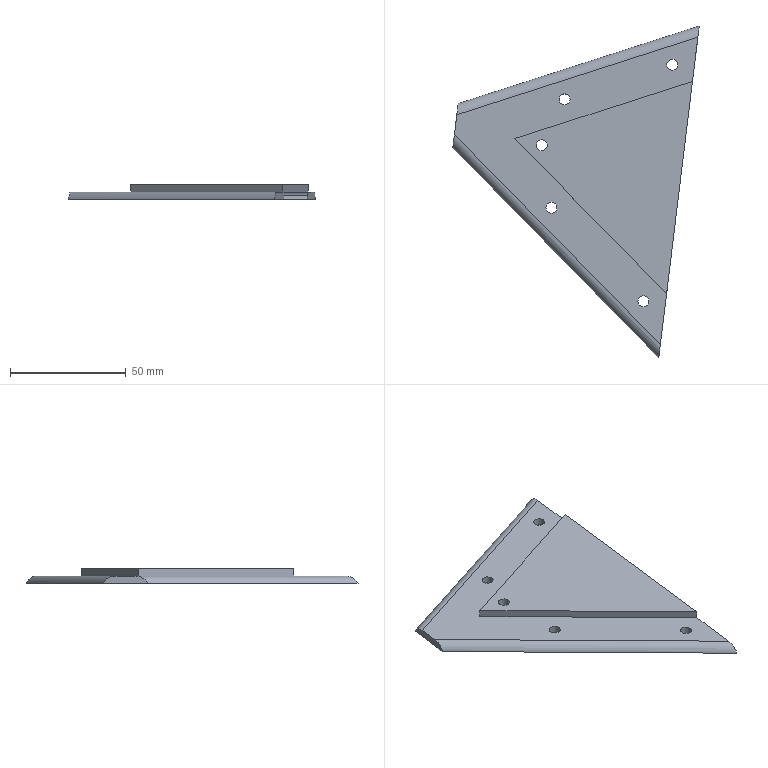Part | NX | features MG0301 nose pivot 24(left) 2 | 1 solid | 25 faces | box 106.679 x 143.723 x 6.35 mm | volume 27507 mm3 | cylinder 12 | plane 11 | torus 2 | commonest cylinder face diameters 4.763 x5 3.15 x3 9.525 x2 12.7 x2
STEP:
#1=CARTESIAN_POINT('',(-353.678,-108.911,-6.35));
#2=VERTEX_POINT('',#1);
#3=CARTESIAN_POINT('',(-354.276,-113.821,-3.175));
#4=VERTEX_POINT('',#3);
#5=CARTESIAN_POINT('',(-354.276,-113.821,-7.938));
#6=DIRECTION('',(-0.9927,0.1209,0.));
#7=DIRECTION('',(0.1209,0.9927,0.));
#8=AXIS2_PLACEMENT_3D('',#5,#6,#7);
#9=ELLIPSE('',#8,5.246,4.763);
#10=EDGE_CURVE('',#2,#4,#9,.F.);
#11=ORIENTED_EDGE('',*,*,#10,.F.);
#12=CARTESIAN_POINT('',(-356.021,-128.145,-6.35));
#13=VERTEX_POINT('',#12);
#14=CARTESIAN_POINT('',(-353.219,-105.142,-6.35));
#15=DIRECTION('',(-0.1209,-0.9927,0.));
#16=VECTOR('',#15,1000.);
#17=LINE('',#14,#16);
#18=EDGE_CURVE('',#2,#13,#17,.T.);
#19=ORIENTED_EDGE('',*,*,#18,.T.);
#20=CARTESIAN_POINT('',(-355.326,-122.441,-3.175));
#21=VERTEX_POINT('',#20);
#22=CARTESIAN_POINT('',(-355.326,-122.441,-7.938));
#23=DIRECTION('',(-0.9927,0.1209,0.));
#24=DIRECTION('',(0.1209,0.9927,0.));
#25=AXIS2_PLACEMENT_3D('',#22,#23,#24);
#26=ELLIPSE('',#25,6.095,4.763);
#27=EDGE_CURVE('',#21,#13,#26,.F.);
#28=ORIENTED_EDGE('',*,*,#27,.F.);
#29=CARTESIAN_POINT('',(-353.219,-105.142,-3.175));
#30=DIRECTION('',(-0.1209,-0.9927,0.));
#31=VECTOR('',#30,1000.);
#32=LINE('',#29,#31);
#33=EDGE_CURVE('',#4,#21,#32,.T.);
#34=ORIENTED_EDGE('',*,*,#33,.F.);
#35=EDGE_LOOP('',(#11,#19,#28,#34));
#36=FACE_BOUND('',#35,.T.);
#37=CARTESIAN_POINT('',(-353.219,-105.142,-6.35));
#38=DIRECTION('',(-0.9927,0.1209,0.));
#39=DIRECTION('',(-0.1209,-0.9927,0.));
#40=AXIS2_PLACEMENT_3D('',#37,#38,#39);
#41=PLANE('',#40);
#42=ADVANCED_FACE('',(#36),#41,.T.);
#43=CARTESIAN_POINT('',(-249.941,-80.241,-3.175));
#44=VERTEX_POINT('',#43);
#45=CARTESIAN_POINT('',(-249.343,-75.332,-6.35));
#46=VERTEX_POINT('',#45);
#47=CARTESIAN_POINT('',(-249.941,-80.241,-7.938));
#48=DIRECTION('',(0.9927,-0.1209,0.));
#49=DIRECTION('',(0.1209,0.9927,0.));
#50=AXIS2_PLACEMENT_3D('',#47,#48,#49);
#51=ELLIPSE('',#50,5.246,4.763);
#52=EDGE_CURVE('',#44,#46,#51,.F.);
#53=ORIENTED_EDGE('',*,*,#52,.F.);
#54=CARTESIAN_POINT('',(-252.267,-99.334,-3.175));
#55=VERTEX_POINT('',#54);
#56=CARTESIAN_POINT('',(-248.883,-71.562,-3.175));
#57=DIRECTION('',(0.1209,0.9927,0.));
#58=VECTOR('',#57,1000.);
#59=LINE('',#56,#58);
#60=EDGE_CURVE('',#55,#44,#59,.T.);
#61=ORIENTED_EDGE('',*,*,#60,.F.);
#62=CARTESIAN_POINT('',(-252.267,-99.334,0.));
#63=VERTEX_POINT('',#62);
#64=CARTESIAN_POINT('',(-252.267,-99.334,-6.35));
#65=DIRECTION('',(0.,0.,-1.));
#66=VECTOR('',#65,1000.);
#67=LINE('',#64,#66);
#68=EDGE_CURVE('',#63,#55,#67,.T.);
#69=ORIENTED_EDGE('',*,*,#68,.F.);
#70=CARTESIAN_POINT('',(-263.456,-191.168,0.));
#71=VERTEX_POINT('',#70);
#72=CARTESIAN_POINT('',(-248.883,-71.562,0.));
#73=DIRECTION('',(0.1209,0.9927,0.));
#74=VECTOR('',#73,1000.);
#75=LINE('',#72,#74);
#76=EDGE_CURVE('',#71,#63,#75,.T.);
#77=ORIENTED_EDGE('',*,*,#76,.F.);
#78=CARTESIAN_POINT('',(-263.456,-191.168,-3.175));
#79=VERTEX_POINT('',#78);
#80=CARTESIAN_POINT('',(-263.456,-191.168,-6.35));
#81=DIRECTION('',(0.,0.,1.));
#82=VECTOR('',#81,1000.);
#83=LINE('',#80,#82);
#84=EDGE_CURVE('',#79,#71,#83,.T.);
#85=ORIENTED_EDGE('',*,*,#84,.F.);
#86=CARTESIAN_POINT('',(-266.158,-213.351,-3.175));
#87=VERTEX_POINT('',#86);
#88=CARTESIAN_POINT('',(-248.883,-71.562,-3.175));
#89=DIRECTION('',(0.1209,0.9927,0.));
#90=VECTOR('',#89,1000.);
#91=LINE('',#88,#90);
#92=EDGE_CURVE('',#87,#79,#91,.T.);
#93=ORIENTED_EDGE('',*,*,#92,.F.);
#94=CARTESIAN_POINT('',(-266.853,-219.055,-6.35));
#95=VERTEX_POINT('',#94);
#96=CARTESIAN_POINT('',(-266.158,-213.351,-7.938));
#97=DIRECTION('',(0.9927,-0.1209,0.));
#98=DIRECTION('',(0.1209,0.9927,0.));
#99=AXIS2_PLACEMENT_3D('',#96,#97,#98);
#100=ELLIPSE('',#99,6.095,4.763);
#101=EDGE_CURVE('',#95,#87,#100,.F.);
#102=ORIENTED_EDGE('',*,*,#101,.F.);
#103=CARTESIAN_POINT('',(-262.964,-187.135,-6.35));
#104=VERTEX_POINT('',#103);
#105=CARTESIAN_POINT('',(-248.883,-71.562,-6.35));
#106=DIRECTION('',(0.1209,0.9927,0.));
#107=VECTOR('',#106,1000.);
#108=LINE('',#105,#107);
#109=EDGE_CURVE('',#95,#104,#108,.T.);
#110=ORIENTED_EDGE('',*,*,#109,.T.);
#111=CARTESIAN_POINT('',(-262.964,-187.135,-4.75));
#112=VERTEX_POINT('',#111);
#113=CARTESIAN_POINT('',(-262.964,-187.135,-22.225));
#114=DIRECTION('',(0.,0.,1.));
#115=VECTOR('',#114,1000.);
#116=LINE('',#113,#115);
#117=EDGE_CURVE('',#104,#112,#116,.T.);
#118=ORIENTED_EDGE('',*,*,#117,.T.);
#119=CARTESIAN_POINT('',(-262.721,-185.135,-3.175));
#120=VERTEX_POINT('',#119);
#121=CARTESIAN_POINT('',(-262.721,-185.135,-4.75));
#122=DIRECTION('',(0.9927,-0.1209,0.));
#123=DIRECTION('',(-0.1209,-0.9927,0.));
#124=AXIS2_PLACEMENT_3D('',#121,#122,#123);
#125=ELLIPSE('',#124,2.015,1.575);
#126=EDGE_CURVE('',#112,#120,#125,.F.);
#127=ORIENTED_EDGE('',*,*,#126,.T.);
#128=CARTESIAN_POINT('',(-252.9,-104.528,-3.175));
#129=VERTEX_POINT('',#128);
#130=CARTESIAN_POINT('',(-252.69,-102.806,-3.175));
#131=DIRECTION('',(0.1209,0.9927,0.));
#132=VECTOR('',#131,1000.);
#133=LINE('',#130,#132);
#134=EDGE_CURVE('',#120,#129,#133,.T.);
#135=ORIENTED_EDGE('',*,*,#134,.T.);
#136=CARTESIAN_POINT('',(-252.69,-102.806,-4.75));
#137=VERTEX_POINT('',#136);
#138=CARTESIAN_POINT('',(-252.9,-104.528,-4.75));
#139=DIRECTION('',(0.9927,-0.1209,0.));
#140=DIRECTION('',(-0.1209,-0.9927,0.));
#141=AXIS2_PLACEMENT_3D('',#138,#139,#140);
#142=ELLIPSE('',#141,1.735,1.575);
#143=EDGE_CURVE('',#129,#137,#142,.F.);
#144=ORIENTED_EDGE('',*,*,#143,.T.);
#145=CARTESIAN_POINT('',(-252.69,-102.806,-6.35));
#146=VERTEX_POINT('',#145);
#147=CARTESIAN_POINT('',(-252.69,-102.806,-22.225));
#148=DIRECTION('',(0.,0.,1.));
#149=VECTOR('',#148,1000.);
#150=LINE('',#147,#149);
#151=EDGE_CURVE('',#146,#137,#150,.T.);
#152=ORIENTED_EDGE('',*,*,#151,.F.);
#153=CARTESIAN_POINT('',(-248.883,-71.562,-6.35));
#154=DIRECTION('',(0.1209,0.9927,0.));
#155=VECTOR('',#154,1000.);
#156=LINE('',#153,#155);
#157=EDGE_CURVE('',#146,#46,#156,.T.);
#158=ORIENTED_EDGE('',*,*,#157,.T.);
#159=EDGE_LOOP('',(#53,#61,#69,#77,#85,#93,#102,#110,#118,#127,#135,#144,#152,#158));
#160=FACE_BOUND('',#159,.T.);
#161=CARTESIAN_POINT('',(-248.883,-71.562,-6.35));
#162=DIRECTION('',(0.9927,-0.1209,0.));
#163=DIRECTION('',(0.1209,0.9927,0.));
#164=AXIS2_PLACEMENT_3D('',#161,#162,#163);
#165=PLANE('',#164);
#166=ADVANCED_FACE('',(#160),#165,.T.);
#167=CARTESIAN_POINT('',(-305.21,-107.134,-6.35));
#168=VERTEX_POINT('',#167);
#169=CARTESIAN_POINT('',(-307.591,-107.134,-6.35));
#170=DIRECTION('',(0.,0.,1.));
#171=DIRECTION('',(1.,0.,0.));
#172=AXIS2_PLACEMENT_3D('',#169,#170,#171);
#173=CIRCLE('',#172,2.381);
#174=EDGE_CURVE('',#168,#168,#173,.T.);
#175=ORIENTED_EDGE('',*,*,#174,.T.);
#176=EDGE_LOOP('',(#175));
#177=FACE_BOUND('',#176,.T.);
#178=CARTESIAN_POINT('',(-258.604,-92.134,-6.35));
#179=VERTEX_POINT('',#178);
#180=CARTESIAN_POINT('',(-260.985,-92.134,-6.35));
#181=DIRECTION('',(0.,0.,1.));
#182=DIRECTION('',(1.,0.,0.));
#183=AXIS2_PLACEMENT_3D('',#180,#181,#182);
#184=CIRCLE('',#183,2.381);
#185=EDGE_CURVE('',#179,#179,#184,.T.);
#186=ORIENTED_EDGE('',*,*,#185,.T.);
#187=EDGE_LOOP('',(#186));
#188=FACE_BOUND('',#187,.T.);
#189=CARTESIAN_POINT('',(-310.915,-153.957,-6.35));
#190=VERTEX_POINT('',#189);
#191=CARTESIAN_POINT('',(-313.296,-153.957,-6.35));
#192=DIRECTION('',(0.,0.,1.));
#193=DIRECTION('',(1.,0.,0.));
#194=AXIS2_PLACEMENT_3D('',#191,#192,#193);
#195=CIRCLE('',#194,2.381);
#196=EDGE_CURVE('',#190,#190,#195,.T.);
#197=ORIENTED_EDGE('',*,*,#196,.T.);
#198=EDGE_LOOP('',(#197));
#199=FACE_BOUND('',#198,.T.);
#200=CARTESIAN_POINT('',(-271.084,-194.566,-6.35));
#201=VERTEX_POINT('',#200);
#202=CARTESIAN_POINT('',(-273.465,-194.566,-6.35));
#203=DIRECTION('',(0.,0.,1.));
#204=DIRECTION('',(1.,0.,0.));
#205=AXIS2_PLACEMENT_3D('',#202,#203,#204);
#206=CIRCLE('',#205,2.381);
#207=EDGE_CURVE('',#201,#201,#206,.T.);
#208=ORIENTED_EDGE('',*,*,#207,.T.);
#209=EDGE_LOOP('',(#208));
#210=FACE_BOUND('',#209,.T.);
#211=CARTESIAN_POINT('',(-315.119,-127.,-6.35));
#212=VERTEX_POINT('',#211);
#213=CARTESIAN_POINT('',(-317.5,-127.,-6.35));
#214=DIRECTION('',(0.,0.,1.));
#215=DIRECTION('',(1.,0.,0.));
#216=AXIS2_PLACEMENT_3D('',#213,#214,#215);
#217=CIRCLE('',#216,2.381);
#218=EDGE_CURVE('',#212,#212,#217,.T.);
#219=ORIENTED_EDGE('',*,*,#218,.T.);
#220=EDGE_LOOP('',(#219));
#221=FACE_BOUND('',#220,.T.);
#222=ORIENTED_EDGE('',*,*,#18,.F.);
#223=CARTESIAN_POINT('',(-475.205,-148.024,-6.35));
#224=DIRECTION('',(0.9519,0.3064,0.));
#225=VECTOR('',#224,1000.);
#226=LINE('',#223,#225);
#227=EDGE_CURVE('',#2,#46,#226,.T.);
#228=ORIENTED_EDGE('',*,*,#227,.T.);
#229=ORIENTED_EDGE('',*,*,#157,.F.);
#230=CARTESIAN_POINT('',(-295.429,-116.561,-6.35));
#231=VERTEX_POINT('',#230);
#232=CARTESIAN_POINT('',(-344.464,-132.343,-6.35));
#233=DIRECTION('',(-0.9519,-0.3064,0.));
#234=VECTOR('',#233,1000.);
#235=LINE('',#232,#234);
#236=EDGE_CURVE('',#146,#231,#235,.T.);
#237=ORIENTED_EDGE('',*,*,#236,.T.);
#238=CARTESIAN_POINT('',(-299.787,-121.838,-6.35));
#239=VERTEX_POINT('',#238);
#240=CARTESIAN_POINT('',(-293.484,-122.606,-6.35));
#241=DIRECTION('',(0.,0.,1.));
#242=DIRECTION('',(1.,0.,0.));
#243=AXIS2_PLACEMENT_3D('',#240,#241,#242);
#244=CIRCLE('',#243,6.35);
#245=EDGE_CURVE('',#231,#239,#244,.T.);
#246=ORIENTED_EDGE('',*,*,#245,.T.);
#247=CARTESIAN_POINT('',(-302.426,-143.493,-6.35));
#248=VERTEX_POINT('',#247);
#249=CARTESIAN_POINT('',(-298.565,-111.801,-6.35));
#250=DIRECTION('',(-0.1209,-0.9927,0.));
#251=VECTOR('',#250,1000.);
#252=LINE('',#249,#251);
#253=EDGE_CURVE('',#239,#248,#252,.T.);
#254=ORIENTED_EDGE('',*,*,#253,.T.);
#255=CARTESIAN_POINT('',(-300.656,-148.708,-6.35));
#256=VERTEX_POINT('',#255);
#257=CARTESIAN_POINT('',(-296.122,-144.261,-6.35));
#258=DIRECTION('',(0.,0.,1.));
#259=DIRECTION('',(1.,0.,0.));
#260=AXIS2_PLACEMENT_3D('',#257,#258,#259);
#261=CIRCLE('',#260,6.35);
#262=EDGE_CURVE('',#248,#256,#261,.T.);
#263=ORIENTED_EDGE('',*,*,#262,.T.);
#264=CARTESIAN_POINT('',(-348.207,-100.227,-6.35));
#265=DIRECTION('',(0.7002,-0.7139,0.));
#266=VECTOR('',#265,1000.);
#267=LINE('',#264,#266);
#268=EDGE_CURVE('',#256,#104,#267,.T.);
#269=ORIENTED_EDGE('',*,*,#268,.T.);
#270=ORIENTED_EDGE('',*,*,#109,.F.);
#271=CARTESIAN_POINT('',(22.703,-514.268,-6.35));
#272=DIRECTION('',(-0.7002,0.7139,0.));
#273=VECTOR('',#272,1000.);
#274=LINE('',#271,#273);
#275=EDGE_CURVE('',#95,#13,#274,.T.);
#276=ORIENTED_EDGE('',*,*,#275,.T.);
#277=EDGE_LOOP('',(#222,#228,#229,#237,#246,#254,#263,#269,#270,#276));
#278=FACE_BOUND('',#277,.T.);
#279=CARTESIAN_POINT('',(-353.219,-105.142,-6.35));
#280=DIRECTION('',(0.,0.,1.));
#281=DIRECTION('',(1.,0.,0.));
#282=AXIS2_PLACEMENT_3D('',#279,#280,#281);
#283=PLANE('',#282);
#284=ADVANCED_FACE('',(#177,#188,#199,#210,#221,#278),#283,.F.);
#285=CARTESIAN_POINT('',(-329.234,-124.106,0.));
#286=VERTEX_POINT('',#285);
#287=CARTESIAN_POINT('',(-468.479,-168.921,0.));
#288=DIRECTION('',(0.9519,0.3064,0.));
#289=VECTOR('',#288,1000.);
#290=LINE('',#287,#289);
#291=EDGE_CURVE('',#286,#63,#290,.T.);
#292=ORIENTED_EDGE('',*,*,#291,.F.);
#293=CARTESIAN_POINT('',(-350.474,-102.45,0.));
#294=DIRECTION('',(-0.7002,0.7139,0.));
#295=VECTOR('',#294,1000.);
#296=LINE('',#293,#295);
#297=EDGE_CURVE('',#71,#286,#296,.T.);
#298=ORIENTED_EDGE('',*,*,#297,.F.);
#299=ORIENTED_EDGE('',*,*,#76,.T.);
#300=EDGE_LOOP('',(#292,#298,#299));
#301=FACE_BOUND('',#300,.T.);
#302=CARTESIAN_POINT('',(-315.119,-127.,0.));
#303=VERTEX_POINT('',#302);
#304=CARTESIAN_POINT('',(-317.5,-127.,0.));
#305=DIRECTION('',(0.,0.,1.));
#306=DIRECTION('',(1.,0.,0.));
#307=AXIS2_PLACEMENT_3D('',#304,#305,#306);
#308=CIRCLE('',#307,2.381);
#309=EDGE_CURVE('',#303,#303,#308,.T.);
#310=ORIENTED_EDGE('',*,*,#309,.F.);
#311=EDGE_LOOP('',(#310));
#312=FACE_BOUND('',#311,.T.);
#313=CARTESIAN_POINT('',(-353.219,-105.142,0.));
#314=DIRECTION('',(0.,0.,1.));
#315=DIRECTION('',(1.,0.,0.));
#316=AXIS2_PLACEMENT_3D('',#313,#314,#315);
#317=PLANE('',#316);
#318=ADVANCED_FACE('',(#301,#312),#317,.T.);
#319=ORIENTED_EDGE('',*,*,#218,.F.);
#320=EDGE_LOOP('',(#319));
#321=FACE_BOUND('',#320,.T.);
#322=ORIENTED_EDGE('',*,*,#309,.T.);
#323=EDGE_LOOP('',(#322));
#324=FACE_BOUND('',#323,.T.);
#325=CARTESIAN_POINT('',(-317.5,-127.,-6.35));
#326=DIRECTION('',(0.,0.,1.));
#327=DIRECTION('',(1.,0.,0.));
#328=AXIS2_PLACEMENT_3D('',#325,#326,#327);
#329=CYLINDRICAL_SURFACE('',#328,2.381);
#330=ADVANCED_FACE('',(#321,#324),#329,.F.);
#331=CARTESIAN_POINT('',(-300.656,-148.708,-4.75));
#332=VERTEX_POINT('',#331);
#333=CARTESIAN_POINT('',(-300.656,-148.708,-3.175));
#334=DIRECTION('',(0.,0.,1.));
#335=VECTOR('',#334,1000.);
#336=LINE('',#333,#335);
#337=EDGE_CURVE('',#256,#332,#336,.T.);
#338=ORIENTED_EDGE('',*,*,#337,.T.);
#339=CARTESIAN_POINT('',(-302.795,-146.526,-4.75));
#340=DIRECTION('',(0.7002,-0.7139,0.));
#341=VECTOR('',#340,1000.);
#342=LINE('',#339,#341);
#343=EDGE_CURVE('',#332,#112,#342,.T.);
#344=ORIENTED_EDGE('',*,*,#343,.T.);
#345=ORIENTED_EDGE('',*,*,#117,.F.);
#346=ORIENTED_EDGE('',*,*,#268,.F.);
#347=EDGE_LOOP('',(#338,#344,#345,#346));
#348=FACE_BOUND('',#347,.T.);
#349=CARTESIAN_POINT('',(-302.795,-146.526,-22.225));
#350=DIRECTION('',(-0.7139,-0.7002,0.));
#351=DIRECTION('',(0.7002,-0.7139,0.));
#352=AXIS2_PLACEMENT_3D('',#349,#350,#351);
#353=PLANE('',#352);
#354=ADVANCED_FACE('',(#348),#353,.F.);
#355=CARTESIAN_POINT('',(-299.787,-121.838,-4.75));
#356=VERTEX_POINT('',#355);
#357=CARTESIAN_POINT('',(-299.787,-121.838,-3.175));
#358=DIRECTION('',(0.,0.,1.));
#359=VECTOR('',#358,1000.);
#360=LINE('',#357,#359);
#361=EDGE_CURVE('',#239,#356,#360,.T.);
#362=ORIENTED_EDGE('',*,*,#361,.T.);
#363=CARTESIAN_POINT('',(-302.426,-143.493,-4.75));
#364=VERTEX_POINT('',#363);
#365=CARTESIAN_POINT('',(-299.296,-117.806,-4.75));
#366=DIRECTION('',(-0.1209,-0.9927,0.));
#367=VECTOR('',#366,1000.);
#368=LINE('',#365,#367);
#369=EDGE_CURVE('',#356,#364,#368,.T.);
#370=ORIENTED_EDGE('',*,*,#369,.T.);
#371=CARTESIAN_POINT('',(-302.426,-143.493,-6.35));
#372=DIRECTION('',(0.,0.,1.));
#373=VECTOR('',#372,1000.);
#374=LINE('',#371,#373);
#375=EDGE_CURVE('',#364,#248,#374,.F.);
#376=ORIENTED_EDGE('',*,*,#375,.T.);
#377=ORIENTED_EDGE('',*,*,#253,.F.);
#378=EDGE_LOOP('',(#362,#370,#376,#377));
#379=FACE_BOUND('',#378,.T.);
#380=CARTESIAN_POINT('',(-299.296,-117.806,-22.225));
#381=DIRECTION('',(-0.9927,0.1209,0.));
#382=DIRECTION('',(-0.1209,-0.9927,0.));
#383=AXIS2_PLACEMENT_3D('',#380,#381,#382);
#384=PLANE('',#383);
#385=ADVANCED_FACE('',(#379),#384,.F.);
#386=ORIENTED_EDGE('',*,*,#151,.T.);
#387=CARTESIAN_POINT('',(-295.429,-116.561,-4.75));
#388=VERTEX_POINT('',#387);
#389=CARTESIAN_POINT('',(-252.69,-102.806,-4.75));
#390=DIRECTION('',(-0.9519,-0.3064,0.));
#391=VECTOR('',#390,1000.);
#392=LINE('',#389,#391);
#393=EDGE_CURVE('',#137,#388,#392,.T.);
#394=ORIENTED_EDGE('',*,*,#393,.T.);
#395=CARTESIAN_POINT('',(-295.429,-116.561,-6.35));
#396=DIRECTION('',(0.,0.,1.));
#397=VECTOR('',#396,1000.);
#398=LINE('',#395,#397);
#399=EDGE_CURVE('',#388,#231,#398,.F.);
#400=ORIENTED_EDGE('',*,*,#399,.T.);
#401=ORIENTED_EDGE('',*,*,#236,.F.);
#402=EDGE_LOOP('',(#386,#394,#400,#401));
#403=FACE_BOUND('',#402,.T.);
#404=CARTESIAN_POINT('',(-252.69,-102.806,-22.225));
#405=DIRECTION('',(-0.3064,0.9519,0.));
#406=DIRECTION('',(-0.9519,-0.3064,0.));
#407=AXIS2_PLACEMENT_3D('',#404,#405,#406);
#408=PLANE('',#407);
#409=ADVANCED_FACE('',(#403),#408,.F.);
#410=ORIENTED_EDGE('',*,*,#134,.F.);
#411=CARTESIAN_POINT('',(-299.531,-147.605,-3.175));
#412=VERTEX_POINT('',#411);
#413=CARTESIAN_POINT('',(-298.959,-148.188,-3.175));
#414=DIRECTION('',(0.7002,-0.7139,0.));
#415=VECTOR('',#414,1000.);
#416=LINE('',#413,#415);
#417=EDGE_CURVE('',#120,#412,#416,.F.);
#418=ORIENTED_EDGE('',*,*,#417,.T.);
#419=CARTESIAN_POINT('',(-300.863,-143.684,-3.175));
#420=VERTEX_POINT('',#419);
#421=CARTESIAN_POINT('',(-296.122,-144.261,-3.175));
#422=DIRECTION('',(0.,0.,-1.));
#423=DIRECTION('',(-1.,0.,0.));
#424=AXIS2_PLACEMENT_3D('',#421,#422,#423);
#425=CIRCLE('',#424,4.775);
#426=EDGE_CURVE('',#412,#420,#425,.T.);
#427=ORIENTED_EDGE('',*,*,#426,.T.);
#428=CARTESIAN_POINT('',(-298.224,-122.028,-3.175));
#429=VERTEX_POINT('',#428);
#430=CARTESIAN_POINT('',(-295.25,-97.62,-3.175));
#431=DIRECTION('',(-0.1209,-0.9927,0.));
#432=VECTOR('',#431,1000.);
#433=LINE('',#430,#432);
#434=EDGE_CURVE('',#420,#429,#433,.F.);
#435=ORIENTED_EDGE('',*,*,#434,.T.);
#436=CARTESIAN_POINT('',(-294.947,-118.06,-3.175));
#437=VERTEX_POINT('',#436);
#438=CARTESIAN_POINT('',(-293.484,-122.606,-3.175));
#439=DIRECTION('',(0.,0.,-1.));
#440=DIRECTION('',(-1.,0.,0.));
#441=AXIS2_PLACEMENT_3D('',#438,#439,#440);
#442=CIRCLE('',#441,4.775);
#443=EDGE_CURVE('',#429,#437,#442,.T.);
#444=ORIENTED_EDGE('',*,*,#443,.T.);
#445=CARTESIAN_POINT('',(-252.207,-104.305,-3.175));
#446=DIRECTION('',(-0.9519,-0.3064,0.));
#447=VECTOR('',#446,1000.);
#448=LINE('',#445,#447);
#449=EDGE_CURVE('',#437,#129,#448,.F.);
#450=ORIENTED_EDGE('',*,*,#449,.T.);
#451=EDGE_LOOP('',(#410,#418,#427,#435,#444,#450));
#452=FACE_BOUND('',#451,.T.);
#453=CARTESIAN_POINT('',(-252.69,-102.806,-3.175));
#454=DIRECTION('',(0.,0.,-1.));
#455=DIRECTION('',(-1.,0.,0.));
#456=AXIS2_PLACEMENT_3D('',#453,#454,#455);
#457=PLANE('',#456);
#458=ADVANCED_FACE('',(#452),#457,.T.);
#459=ORIENTED_EDGE('',*,*,#375,.F.);
#460=CARTESIAN_POINT('',(-296.122,-144.261,-4.75));
#461=DIRECTION('',(0.,0.,-1.));
#462=DIRECTION('',(-1.,0.,0.));
#463=AXIS2_PLACEMENT_3D('',#460,#461,#462);
#464=CIRCLE('',#463,6.35);
#465=EDGE_CURVE('',#364,#332,#464,.F.);
#466=ORIENTED_EDGE('',*,*,#465,.T.);
#467=ORIENTED_EDGE('',*,*,#337,.F.);
#468=ORIENTED_EDGE('',*,*,#262,.F.);
#469=EDGE_LOOP('',(#459,#466,#467,#468));
#470=FACE_BOUND('',#469,.T.);
#471=CARTESIAN_POINT('',(-296.122,-144.261,-22.225));
#472=DIRECTION('',(0.,0.,-1.));
#473=DIRECTION('',(-1.,0.,0.));
#474=AXIS2_PLACEMENT_3D('',#471,#472,#473);
#475=CYLINDRICAL_SURFACE('',#474,6.35);
#476=ADVANCED_FACE('',(#470),#475,.F.);
#477=ORIENTED_EDGE('',*,*,#399,.F.);
#478=CARTESIAN_POINT('',(-293.484,-122.606,-4.75));
#479=DIRECTION('',(0.,0.,-1.));
#480=DIRECTION('',(-1.,0.,0.));
#481=AXIS2_PLACEMENT_3D('',#478,#479,#480);
#482=CIRCLE('',#481,6.35);
#483=EDGE_CURVE('',#388,#356,#482,.F.);
#484=ORIENTED_EDGE('',*,*,#483,.T.);
#485=ORIENTED_EDGE('',*,*,#361,.F.);
#486=ORIENTED_EDGE('',*,*,#245,.F.);
#487=EDGE_LOOP('',(#477,#484,#485,#486));
#488=FACE_BOUND('',#487,.T.);
#489=CARTESIAN_POINT('',(-293.484,-122.606,-22.225));
#490=DIRECTION('',(0.,0.,-1.));
#491=DIRECTION('',(-1.,0.,0.));
#492=AXIS2_PLACEMENT_3D('',#489,#490,#491);
#493=CYLINDRICAL_SURFACE('',#492,6.35);
#494=ADVANCED_FACE('',(#488),#493,.F.);
#495=ORIENTED_EDGE('',*,*,#27,.T.);
#496=ORIENTED_EDGE('',*,*,#275,.F.);
#497=ORIENTED_EDGE('',*,*,#101,.T.);
#498=CARTESIAN_POINT('',(25.908,-511.124,-3.175));
#499=DIRECTION('',(-0.7002,0.7139,0.));
#500=VECTOR('',#499,1000.);
#501=LINE('',#498,#500);
#502=EDGE_CURVE('',#87,#21,#501,.T.);
#503=ORIENTED_EDGE('',*,*,#502,.T.);
#504=EDGE_LOOP('',(#495,#496,#497,#503));
#505=FACE_BOUND('',#504,.T.);
#506=CARTESIAN_POINT('',(25.908,-511.124,-7.938));
#507=DIRECTION('',(-0.7002,0.7139,0.));
#508=DIRECTION('',(-0.7139,-0.7002,0.));
#509=AXIS2_PLACEMENT_3D('',#506,#507,#508);
#510=CYLINDRICAL_SURFACE('',#509,4.763);
#511=ADVANCED_FACE('',(#505),#510,.T.);
#512=CARTESIAN_POINT('',(-309.973,-107.134,-3.175));
#513=VERTEX_POINT('',#512);
#514=CARTESIAN_POINT('',(-307.591,-107.134,-3.175));
#515=DIRECTION('',(0.,0.,-1.));
#516=DIRECTION('',(-1.,0.,0.));
#517=AXIS2_PLACEMENT_3D('',#514,#515,#516);
#518=CIRCLE('',#517,2.381);
#519=EDGE_CURVE('',#513,#513,#518,.T.);
#520=ORIENTED_EDGE('',*,*,#519,.T.);
#521=EDGE_LOOP('',(#520));
#522=FACE_BOUND('',#521,.T.);
#523=CARTESIAN_POINT('',(-263.366,-92.134,-3.175));
#524=VERTEX_POINT('',#523);
#525=CARTESIAN_POINT('',(-260.985,-92.134,-3.175));
#526=DIRECTION('',(0.,0.,-1.));
#527=DIRECTION('',(-1.,0.,0.));
#528=AXIS2_PLACEMENT_3D('',#525,#526,#527);
#529=CIRCLE('',#528,2.381);
#530=EDGE_CURVE('',#524,#524,#529,.T.);
#531=ORIENTED_EDGE('',*,*,#530,.T.);
#532=EDGE_LOOP('',(#531));
#533=FACE_BOUND('',#532,.T.);
#534=CARTESIAN_POINT('',(-315.677,-153.957,-3.175));
#535=VERTEX_POINT('',#534);
#536=CARTESIAN_POINT('',(-313.296,-153.957,-3.175));
#537=DIRECTION('',(0.,0.,-1.));
#538=DIRECTION('',(-1.,0.,0.));
#539=AXIS2_PLACEMENT_3D('',#536,#537,#538);
#540=CIRCLE('',#539,2.381);
#541=EDGE_CURVE('',#535,#535,#540,.T.);
#542=ORIENTED_EDGE('',*,*,#541,.T.);
#543=EDGE_LOOP('',(#542));
#544=FACE_BOUND('',#543,.T.);
#545=CARTESIAN_POINT('',(-275.846,-194.566,-3.175));
#546=VERTEX_POINT('',#545);
#547=CARTESIAN_POINT('',(-273.465,-194.566,-3.175));
#548=DIRECTION('',(0.,0.,-1.));
#549=DIRECTION('',(-1.,0.,0.));
#550=AXIS2_PLACEMENT_3D('',#547,#548,#549);
#551=CIRCLE('',#550,2.381);
#552=EDGE_CURVE('',#546,#546,#551,.T.);
#553=ORIENTED_EDGE('',*,*,#552,.T.);
#554=EDGE_LOOP('',(#553));
#555=FACE_BOUND('',#554,.T.);
#556=CARTESIAN_POINT('',(-329.234,-124.106,-3.175));
#557=VERTEX_POINT('',#556);
#558=CARTESIAN_POINT('',(38.375,-498.896,-3.175));
#559=DIRECTION('',(-0.7002,0.7139,0.));
#560=VECTOR('',#559,1000.);
#561=LINE('',#558,#560);
#562=EDGE_CURVE('',#79,#557,#561,.T.);
#563=ORIENTED_EDGE('',*,*,#562,.T.);
#564=CARTESIAN_POINT('',(-468.479,-168.921,-3.175));
#565=DIRECTION('',(0.9519,0.3064,0.));
#566=VECTOR('',#565,1000.);
#567=LINE('',#564,#566);
#568=EDGE_CURVE('',#557,#55,#567,.T.);
#569=ORIENTED_EDGE('',*,*,#568,.T.);
#570=ORIENTED_EDGE('',*,*,#60,.T.);
#571=CARTESIAN_POINT('',(-473.829,-152.298,-3.175));
#572=DIRECTION('',(0.9519,0.3064,0.));
#573=VECTOR('',#572,1000.);
#574=LINE('',#571,#573);
#575=EDGE_CURVE('',#4,#44,#574,.T.);
#576=ORIENTED_EDGE('',*,*,#575,.F.);
#577=ORIENTED_EDGE('',*,*,#33,.T.);
#578=ORIENTED_EDGE('',*,*,#502,.F.);
#579=ORIENTED_EDGE('',*,*,#92,.T.);
#580=EDGE_LOOP('',(#563,#569,#570,#576,#577,#578,#579));
#581=FACE_BOUND('',#580,.T.);
#582=CARTESIAN_POINT('',(38.375,-498.896,-3.175));
#583=DIRECTION('',(0.,0.,-1.));
#584=DIRECTION('',(-1.,0.,0.));
#585=AXIS2_PLACEMENT_3D('',#582,#583,#584);
#586=PLANE('',#585);
#587=ADVANCED_FACE('',(#522,#533,#544,#555,#581),#586,.F.);
#588=ORIENTED_EDGE('',*,*,#297,.T.);
#589=CARTESIAN_POINT('',(-329.234,-124.106,0.));
#590=DIRECTION('',(0.,0.,-1.));
#591=VECTOR('',#590,1000.);
#592=LINE('',#589,#591);
#593=EDGE_CURVE('',#286,#557,#592,.T.);
#594=ORIENTED_EDGE('',*,*,#593,.T.);
#595=ORIENTED_EDGE('',*,*,#562,.F.);
#596=ORIENTED_EDGE('',*,*,#84,.T.);
#597=EDGE_LOOP('',(#588,#594,#595,#596));
#598=FACE_BOUND('',#597,.T.);
#599=CARTESIAN_POINT('',(38.375,-498.896,0.));
#600=DIRECTION('',(0.7139,0.7002,0.));
#601=DIRECTION('',(-0.7002,0.7139,0.));
#602=AXIS2_PLACEMENT_3D('',#599,#600,#601);
#603=PLANE('',#602);
#604=ADVANCED_FACE('',(#598),#603,.F.);
#605=ORIENTED_EDGE('',*,*,#68,.T.);
#606=ORIENTED_EDGE('',*,*,#568,.F.);
#607=ORIENTED_EDGE('',*,*,#593,.F.);
#608=ORIENTED_EDGE('',*,*,#291,.T.);
#609=EDGE_LOOP('',(#605,#606,#607,#608));
#610=FACE_BOUND('',#609,.T.);
#611=CARTESIAN_POINT('',(-468.479,-168.921,0.));
#612=DIRECTION('',(0.3064,-0.9519,0.));
#613=DIRECTION('',(0.9519,0.3064,0.));
#614=AXIS2_PLACEMENT_3D('',#611,#612,#613);
#615=PLANE('',#614);
#616=ADVANCED_FACE('',(#610),#615,.F.);
#617=ORIENTED_EDGE('',*,*,#10,.T.);
#618=ORIENTED_EDGE('',*,*,#575,.T.);
#619=ORIENTED_EDGE('',*,*,#52,.T.);
#620=ORIENTED_EDGE('',*,*,#227,.F.);
#621=EDGE_LOOP('',(#617,#618,#619,#620));
#622=FACE_BOUND('',#621,.T.);
#623=CARTESIAN_POINT('',(-473.829,-152.298,-7.938));
#624=DIRECTION('',(0.9519,0.3064,0.));
#625=DIRECTION('',(-0.3064,0.9519,0.));
#626=AXIS2_PLACEMENT_3D('',#623,#624,#625);
#627=CYLINDRICAL_SURFACE('',#626,4.763);
#628=ADVANCED_FACE('',(#622),#627,.T.);
#629=ORIENTED_EDGE('',*,*,#143,.F.);
#630=ORIENTED_EDGE('',*,*,#449,.F.);
#631=CARTESIAN_POINT('',(-294.947,-118.06,-4.75));
#632=DIRECTION('',(0.9519,0.3064,0.));
#633=DIRECTION('',(-0.3064,0.9519,0.));
#634=AXIS2_PLACEMENT_3D('',#631,#632,#633);
#635=CIRCLE('',#634,1.575);
#636=EDGE_CURVE('',#388,#437,#635,.T.);
#637=ORIENTED_EDGE('',*,*,#636,.F.);
#638=ORIENTED_EDGE('',*,*,#393,.F.);
#639=EDGE_LOOP('',(#629,#630,#637,#638));
#640=FACE_BOUND('',#639,.T.);
#641=CARTESIAN_POINT('',(-252.207,-104.305,-4.75));
#642=DIRECTION('',(-0.9519,-0.3064,0.));
#643=DIRECTION('',(0.3064,-0.9519,0.));
#644=AXIS2_PLACEMENT_3D('',#641,#642,#643);
#645=CYLINDRICAL_SURFACE('',#644,1.575);
#646=ADVANCED_FACE('',(#640),#645,.F.);
#647=ORIENTED_EDGE('',*,*,#636,.T.);
#648=ORIENTED_EDGE('',*,*,#443,.F.);
#649=CARTESIAN_POINT('',(-298.224,-122.028,-4.75));
#650=DIRECTION('',(0.1209,0.9927,0.));
#651=DIRECTION('',(-0.9927,0.1209,0.));
#652=AXIS2_PLACEMENT_3D('',#649,#650,#651);
#653=CIRCLE('',#652,1.575);
#654=EDGE_CURVE('',#356,#429,#653,.T.);
#655=ORIENTED_EDGE('',*,*,#654,.F.);
#656=ORIENTED_EDGE('',*,*,#483,.F.);
#657=EDGE_LOOP('',(#647,#648,#655,#656));
#658=FACE_BOUND('',#657,.T.);
#659=CARTESIAN_POINT('',(-293.484,-122.606,-4.75));
#660=DIRECTION('',(0.,0.,-1.));
#661=DIRECTION('',(-1.,0.,0.));
#662=AXIS2_PLACEMENT_3D('',#659,#660,#661);
#663=TOROIDAL_SURFACE('',#662,4.775,1.575);
#664=ADVANCED_FACE('',(#658),#663,.F.);
#665=ORIENTED_EDGE('',*,*,#654,.T.);
#666=ORIENTED_EDGE('',*,*,#434,.F.);
#667=CARTESIAN_POINT('',(-300.863,-143.684,-4.75));
#668=DIRECTION('',(0.1209,0.9927,0.));
#669=DIRECTION('',(-0.9927,0.1209,0.));
#670=AXIS2_PLACEMENT_3D('',#667,#668,#669);
#671=CIRCLE('',#670,1.575);
#672=EDGE_CURVE('',#364,#420,#671,.T.);
#673=ORIENTED_EDGE('',*,*,#672,.F.);
#674=ORIENTED_EDGE('',*,*,#369,.F.);
#675=EDGE_LOOP('',(#665,#666,#673,#674));
#676=FACE_BOUND('',#675,.T.);
#677=CARTESIAN_POINT('',(-297.733,-117.996,-4.75));
#678=DIRECTION('',(-0.1209,-0.9927,0.));
#679=DIRECTION('',(0.9927,-0.1209,0.));
#680=AXIS2_PLACEMENT_3D('',#677,#678,#679);
#681=CYLINDRICAL_SURFACE('',#680,1.575);
#682=ADVANCED_FACE('',(#676),#681,.F.);
#683=ORIENTED_EDGE('',*,*,#672,.T.);
#684=ORIENTED_EDGE('',*,*,#426,.F.);
#685=CARTESIAN_POINT('',(-299.531,-147.605,-4.75));
#686=DIRECTION('',(-0.7002,0.7139,0.));
#687=DIRECTION('',(-0.7139,-0.7002,0.));
#688=AXIS2_PLACEMENT_3D('',#685,#686,#687);
#689=CIRCLE('',#688,1.575);
#690=EDGE_CURVE('',#332,#412,#689,.T.);
#691=ORIENTED_EDGE('',*,*,#690,.F.);
#692=ORIENTED_EDGE('',*,*,#465,.F.);
#693=EDGE_LOOP('',(#683,#684,#691,#692));
#694=FACE_BOUND('',#693,.T.);
#695=CARTESIAN_POINT('',(-296.122,-144.261,-4.75));
#696=DIRECTION('',(0.,0.,-1.));
#697=DIRECTION('',(-1.,0.,0.));
#698=AXIS2_PLACEMENT_3D('',#695,#696,#697);
#699=TOROIDAL_SURFACE('',#698,4.775,1.575);
#700=ADVANCED_FACE('',(#694),#699,.F.);
#701=ORIENTED_EDGE('',*,*,#690,.T.);
#702=ORIENTED_EDGE('',*,*,#417,.F.);
#703=ORIENTED_EDGE('',*,*,#126,.F.);
#704=ORIENTED_EDGE('',*,*,#343,.F.);
#705=EDGE_LOOP('',(#701,#702,#703,#704));
#706=FACE_BOUND('',#705,.T.);
#707=CARTESIAN_POINT('',(-301.671,-145.423,-4.75));
#708=DIRECTION('',(0.7002,-0.7139,0.));
#709=DIRECTION('',(0.7139,0.7002,0.));
#710=AXIS2_PLACEMENT_3D('',#707,#708,#709);
#711=CYLINDRICAL_SURFACE('',#710,1.575);
#712=ADVANCED_FACE('',(#706),#711,.F.);
#713=ORIENTED_EDGE('',*,*,#552,.F.);
#714=EDGE_LOOP('',(#713));
#715=FACE_BOUND('',#714,.T.);
#716=ORIENTED_EDGE('',*,*,#207,.F.);
#717=EDGE_LOOP('',(#716));
#718=FACE_BOUND('',#717,.T.);
#719=CARTESIAN_POINT('',(-273.465,-194.566,-63.5));
#720=DIRECTION('',(0.,0.,1.));
#721=DIRECTION('',(1.,0.,0.));
#722=AXIS2_PLACEMENT_3D('',#719,#720,#721);
#723=CYLINDRICAL_SURFACE('',#722,2.381);
#724=ADVANCED_FACE('',(#715,#718),#723,.F.);
#725=ORIENTED_EDGE('',*,*,#541,.F.);
#726=EDGE_LOOP('',(#725));
#727=FACE_BOUND('',#726,.T.);
#728=ORIENTED_EDGE('',*,*,#196,.F.);
#729=EDGE_LOOP('',(#728));
#730=FACE_BOUND('',#729,.T.);
#731=CARTESIAN_POINT('',(-313.296,-153.957,-63.5));
#732=DIRECTION('',(0.,0.,1.));
#733=DIRECTION('',(1.,0.,0.));
#734=AXIS2_PLACEMENT_3D('',#731,#732,#733);
#735=CYLINDRICAL_SURFACE('',#734,2.381);
#736=ADVANCED_FACE('',(#727,#730),#735,.F.);
#737=ORIENTED_EDGE('',*,*,#530,.F.);
#738=EDGE_LOOP('',(#737));
#739=FACE_BOUND('',#738,.T.);
#740=ORIENTED_EDGE('',*,*,#185,.F.);
#741=EDGE_LOOP('',(#740));
#742=FACE_BOUND('',#741,.T.);
#743=CARTESIAN_POINT('',(-260.985,-92.134,-63.5));
#744=DIRECTION('',(0.,0.,1.));
#745=DIRECTION('',(1.,0.,0.));
#746=AXIS2_PLACEMENT_3D('',#743,#744,#745);
#747=CYLINDRICAL_SURFACE('',#746,2.381);
#748=ADVANCED_FACE('',(#739,#742),#747,.F.);
#749=ORIENTED_EDGE('',*,*,#519,.F.);
#750=EDGE_LOOP('',(#749));
#751=FACE_BOUND('',#750,.T.);
#752=ORIENTED_EDGE('',*,*,#174,.F.);
#753=EDGE_LOOP('',(#752));
#754=FACE_BOUND('',#753,.T.);
#755=CARTESIAN_POINT('',(-307.591,-107.134,-63.5));
#756=DIRECTION('',(0.,0.,1.));
#757=DIRECTION('',(1.,0.,0.));
#758=AXIS2_PLACEMENT_3D('',#755,#756,#757);
#759=CYLINDRICAL_SURFACE('',#758,2.381);
#760=ADVANCED_FACE('',(#751,#754),#759,.F.);
#761=CLOSED_SHELL('',(#42,#166,#284,#318,#330,#354,#385,#409,#458,#476,#494,#511,#587,#604,#616,#628,#646,#664,#682,#700,#712,#724,#736,#748,#760));
#762=MANIFOLD_SOLID_BREP('',#761);
#763=(LENGTH_UNIT()NAMED_UNIT(*)SI_UNIT(.MILLI.,.METRE.));
#764=UNCERTAINTY_MEASURE_WITH_UNIT(LENGTH_MEASURE(0.00001),#763,'','');
#765=(NAMED_UNIT(*)PLANE_ANGLE_UNIT()SI_UNIT($,.RADIAN.));
#766=(NAMED_UNIT(*)SI_UNIT($,.STERADIAN.)SOLID_ANGLE_UNIT());
#767=(GEOMETRIC_REPRESENTATION_CONTEXT(3)GLOBAL_UNCERTAINTY_ASSIGNED_CONTEXT((#764))GLOBAL_UNIT_ASSIGNED_CONTEXT((#763,#765,#766))REPRESENTATION_CONTEXT('',''));
#768=ADVANCED_BREP_SHAPE_REPRESENTATION('',(#762),#767);